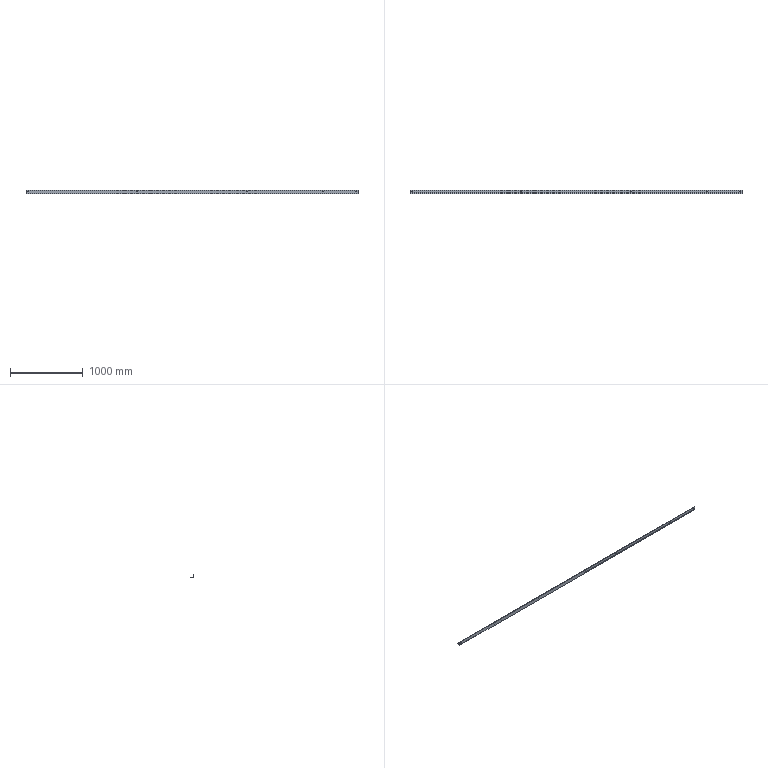Part | STEP file | LINK.ANGLE.stp | 1 solid | 31 faces | box 4550 x 50 x 50 mm | volume 2563197 mm3 | cylinder 15 | spline 8 | plane 8 | commonest cylinder face diameters 10 x12 9 x2 13 x1